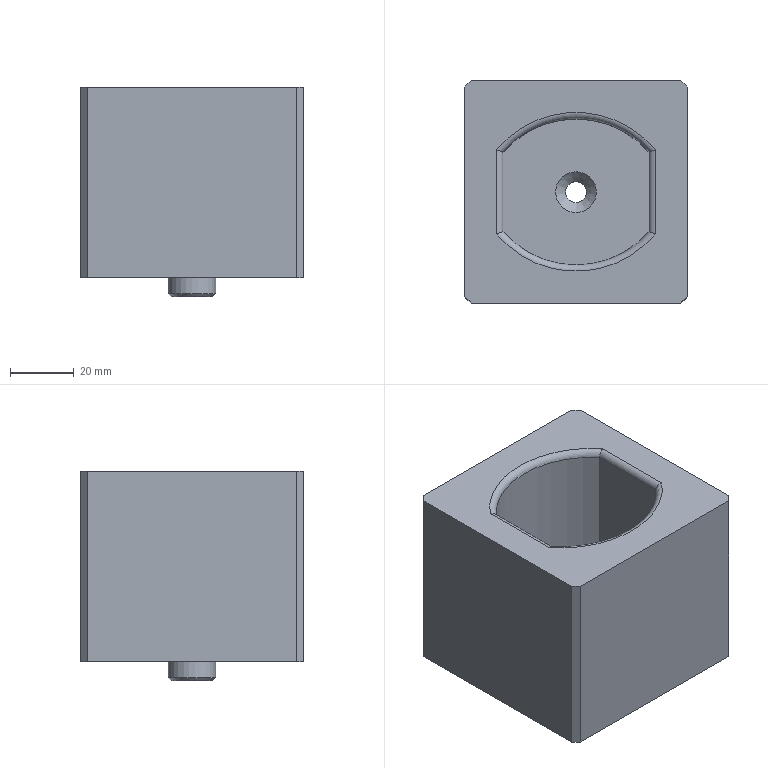NC program | NX | posted with a generic post | part box 70 x 70 x 66 mm
Lines 1 to 58 of 8582:
N10 G17 G21 G94 G90
(FLOOR_WALL_COPY , TOOL : D63)
N12 T01 M6
N14 G54
N16 G17 G0 G90 X-69.5 Y34.997 S6500 M3
N18 G43 Z30. H1
N20 Z6.
N22 G94 G1 Z3. F2500.
N24 X-66.5
N26 X66.5
N28 Y12.599
N30 X-66.5
N32 Y-9.8
N34 X66.5
N36 X69.5
N38 Z6.
N40 G0 Z30.
N42 X-69.5 Y34.997
N44 Z5.
N46 G1 Z2.
N48 X-66.5
N50 X66.5
N52 Y12.599
N54 X-66.5
N56 Y-9.8
N58 X66.5
N60 X69.5
N62 Z5.
N64 G0 Z30.
N66 X-69.5 Y34.997
N68 Z4.
N70 G1 Z1.
N72 X-66.5
N74 X66.5
N76 Y12.599
N78 X-66.5
N80 Y-9.8
N82 X66.5
N84 X69.5
N86 Z4.
N88 G0 Z30.
N90 X-69.5 Y34.997
N92 Z3.
N94 G1 Z0.
N96 X-66.5
N98 X66.5
N100 Y12.599
N102 X-66.5
N104 Y-9.8
N106 X66.5
N108 X69.5
N110 Z3.
N112 G0 Z30.
N114 M5